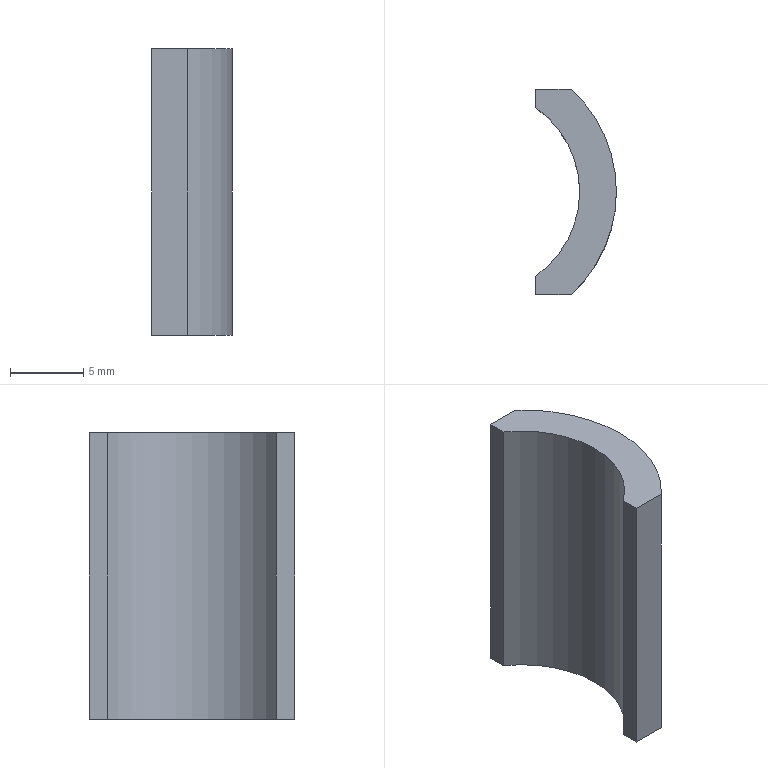Part | STEP file | magnet | 1 solid | 8 faces | box 5.5 x 14 x 19.5 mm | volume 770.904 mm3 | plane 6 | cylinder 2 | commonest cylinder face diameters 14 x1 19 x1
STEP:
#1=CARTESIAN_POINT('',(0.,0.,0.));
#2=DIRECTION('',(0.,0.,1.));
#3=DIRECTION('',(1.,0.,0.));
#4=AXIS2_PLACEMENT_3D('',#1,#2,#3);
#5=CARTESIAN_POINT('',(4.,-7.,0.));
#6=VERTEX_POINT('',#5);
#7=CARTESIAN_POINT('',(6.423,-7.,0.));
#8=VERTEX_POINT('',#7);
#9=CARTESIAN_POINT('',(4.,-7.,0.));
#10=DIRECTION('',(1.,0.,0.));
#11=VECTOR('',#10,1.);
#12=LINE('',#9,#11);
#13=CARTESIAN_POINT('',(4.,-7.,19.5));
#14=DIRECTION('',(0.,1.,0.));
#15=DIRECTION('',(-1.,0.,0.));
#16=AXIS2_PLACEMENT_3D('',#13,#14,#15);
#17=PLANE('',#16);
#18=CARTESIAN_POINT('',(0.,-19.5));
#19=DIRECTION('',(-1.,0.));
#20=VECTOR('',#19,1.);
#21=LINE('',#18,#20);
#22=(GEOMETRIC_REPRESENTATION_CONTEXT(2)PARAMETRIC_REPRESENTATION_CONTEXT()REPRESENTATION_CONTEXT('',''));
#23=DEFINITIONAL_REPRESENTATION('',(#21),#22);
#24=PCURVE('',#17,#23);
#25=CARTESIAN_POINT('',(0.,0.,0.));
#26=DIRECTION('',(0.,0.,1.));
#27=DIRECTION('',(1.,0.,0.));
#28=AXIS2_PLACEMENT_3D('',#25,#26,#27);
#29=PLANE('',#28);
#30=CARTESIAN_POINT('',(4.,-7.));
#31=DIRECTION('',(1.,0.));
#32=VECTOR('',#31,1.);
#33=LINE('',#30,#32);
#34=(GEOMETRIC_REPRESENTATION_CONTEXT(2)PARAMETRIC_REPRESENTATION_CONTEXT()REPRESENTATION_CONTEXT('',''));
#35=DEFINITIONAL_REPRESENTATION('',(#33),#34);
#36=PCURVE('',#29,#35);
#37=SURFACE_CURVE('',#12,(#24,#36),.PCURVE_S1.);
#38=EDGE_CURVE('',#6,#8,#37,.T.);
#39=ORIENTED_EDGE('',*,*,#38,.T.);
#40=CARTESIAN_POINT('',(6.423,-7.,19.5));
#41=VERTEX_POINT('',#40);
#42=CARTESIAN_POINT('',(6.423,-7.,19.5));
#43=DIRECTION('',(0.,0.,-1.));
#44=VECTOR('',#43,1.);
#45=LINE('',#42,#44);
#46=CARTESIAN_POINT('',(-2.423,0.));
#47=DIRECTION('',(0.,-1.));
#48=VECTOR('',#47,1.);
#49=LINE('',#46,#48);
#50=(GEOMETRIC_REPRESENTATION_CONTEXT(2)PARAMETRIC_REPRESENTATION_CONTEXT()REPRESENTATION_CONTEXT('',''));
#51=DEFINITIONAL_REPRESENTATION('',(#49),#50);
#52=PCURVE('',#17,#51);
#53=CARTESIAN_POINT('',(0.,0.,19.5));
#54=DIRECTION('',(0.,0.,-1.));
#55=DIRECTION('',(-1.,0.,0.));
#56=AXIS2_PLACEMENT_3D('',#53,#54,#55);
#57=CYLINDRICAL_SURFACE('',#56,9.5);
#58=CARTESIAN_POINT('',(3.97,0.));
#59=DIRECTION('',(0.,1.));
#60=VECTOR('',#59,1.);
#61=LINE('',#58,#60);
#62=(GEOMETRIC_REPRESENTATION_CONTEXT(2)PARAMETRIC_REPRESENTATION_CONTEXT()REPRESENTATION_CONTEXT('',''));
#63=DEFINITIONAL_REPRESENTATION('',(#61),#62);
#64=PCURVE('',#57,#63);
#65=SURFACE_CURVE('',#45,(#52,#64),.PCURVE_S1.);
#66=EDGE_CURVE('',#41,#8,#65,.T.);
#67=ORIENTED_EDGE('',*,*,#66,.F.);
#68=CARTESIAN_POINT('',(4.,-7.,19.5));
#69=VERTEX_POINT('',#68);
#70=CARTESIAN_POINT('',(4.,-7.,19.5));
#71=DIRECTION('',(1.,0.,0.));
#72=VECTOR('',#71,1.);
#73=LINE('',#70,#72);
#74=CARTESIAN_POINT('',(0.,0.));
#75=DIRECTION('',(-1.,0.));
#76=VECTOR('',#75,1.);
#77=LINE('',#74,#76);
#78=(GEOMETRIC_REPRESENTATION_CONTEXT(2)PARAMETRIC_REPRESENTATION_CONTEXT()REPRESENTATION_CONTEXT('',''));
#79=DEFINITIONAL_REPRESENTATION('',(#77),#78);
#80=PCURVE('',#17,#79);
#81=CARTESIAN_POINT('',(0.,0.,19.5));
#82=DIRECTION('',(0.,0.,1.));
#83=DIRECTION('',(1.,0.,0.));
#84=AXIS2_PLACEMENT_3D('',#81,#82,#83);
#85=PLANE('',#84);
#86=CARTESIAN_POINT('',(4.,-7.));
#87=DIRECTION('',(1.,0.));
#88=VECTOR('',#87,1.);
#89=LINE('',#86,#88);
#90=(GEOMETRIC_REPRESENTATION_CONTEXT(2)PARAMETRIC_REPRESENTATION_CONTEXT()REPRESENTATION_CONTEXT('',''));
#91=DEFINITIONAL_REPRESENTATION('',(#89),#90);
#92=PCURVE('',#85,#91);
#93=SURFACE_CURVE('',#73,(#80,#92),.PCURVE_S1.);
#94=EDGE_CURVE('',#69,#41,#93,.T.);
#95=ORIENTED_EDGE('',*,*,#94,.F.);
#96=CARTESIAN_POINT('',(4.,-7.,19.5));
#97=DIRECTION('',(0.,0.,-1.));
#98=VECTOR('',#97,1.);
#99=LINE('',#96,#98);
#100=CARTESIAN_POINT('',(0.,0.));
#101=DIRECTION('',(0.,-1.));
#102=VECTOR('',#101,1.);
#103=LINE('',#100,#102);
#104=(GEOMETRIC_REPRESENTATION_CONTEXT(2)PARAMETRIC_REPRESENTATION_CONTEXT()REPRESENTATION_CONTEXT('',''));
#105=DEFINITIONAL_REPRESENTATION('',(#103),#104);
#106=PCURVE('',#17,#105);
#107=CARTESIAN_POINT('',(4.,-7.,19.5));
#108=DIRECTION('',(1.,0.,0.));
#109=DIRECTION('',(0.,0.,-1.));
#110=AXIS2_PLACEMENT_3D('',#107,#108,#109);
#111=PLANE('',#110);
#112=CARTESIAN_POINT('',(0.,0.));
#113=DIRECTION('',(1.,0.));
#114=VECTOR('',#113,1.);
#115=LINE('',#112,#114);
#116=(GEOMETRIC_REPRESENTATION_CONTEXT(2)PARAMETRIC_REPRESENTATION_CONTEXT()REPRESENTATION_CONTEXT('',''));
#117=DEFINITIONAL_REPRESENTATION('',(#115),#116);
#118=PCURVE('',#111,#117);
#119=SURFACE_CURVE('',#99,(#106,#118),.PCURVE_S1.);
#120=EDGE_CURVE('',#69,#6,#119,.T.);
#121=ORIENTED_EDGE('',*,*,#120,.T.);
#122=EDGE_LOOP('',(#39,#67,#95,#121));
#123=FACE_BOUND('',#122,.T.);
#124=ADVANCED_FACE('',(#123),#17,.F.);
#125=CARTESIAN_POINT('',(6.423,7.,0.));
#126=VERTEX_POINT('',#125);
#127=CARTESIAN_POINT('',(0.,0.,0.));
#128=DIRECTION('',(0.,0.,1.));
#129=DIRECTION('',(1.,0.,0.));
#130=AXIS2_PLACEMENT_3D('',#127,#128,#129);
#131=CIRCLE('',#130,9.5);
#132=CARTESIAN_POINT('',(9.425,19.5));
#133=DIRECTION('',(-1.,0.));
#134=VECTOR('',#133,1.);
#135=LINE('',#132,#134);
#136=(GEOMETRIC_REPRESENTATION_CONTEXT(2)PARAMETRIC_REPRESENTATION_CONTEXT()REPRESENTATION_CONTEXT('',''));
#137=DEFINITIONAL_REPRESENTATION('',(#135),#136);
#138=PCURVE('',#57,#137);
#139=CARTESIAN_POINT('',(0.,0.));
#140=DIRECTION('',(1.,0.));
#141=AXIS2_PLACEMENT_2D('',#139,#140);
#142=CIRCLE('',#141,9.5);
#143=(GEOMETRIC_REPRESENTATION_CONTEXT(2)PARAMETRIC_REPRESENTATION_CONTEXT()REPRESENTATION_CONTEXT('',''));
#144=DEFINITIONAL_REPRESENTATION('',(#142),#143);
#145=PCURVE('',#29,#144);
#146=SURFACE_CURVE('',#131,(#138,#145),.PCURVE_S1.);
#147=EDGE_CURVE('',#8,#126,#146,.T.);
#148=ORIENTED_EDGE('',*,*,#147,.T.);
#149=CARTESIAN_POINT('',(6.423,7.,19.5));
#150=VERTEX_POINT('',#149);
#151=CARTESIAN_POINT('',(6.423,7.,19.5));
#152=DIRECTION('',(0.,0.,-1.));
#153=VECTOR('',#152,1.);
#154=LINE('',#151,#153);
#155=CARTESIAN_POINT('',(2.313,0.));
#156=DIRECTION('',(0.,1.));
#157=VECTOR('',#156,1.);
#158=LINE('',#155,#157);
#159=(GEOMETRIC_REPRESENTATION_CONTEXT(2)PARAMETRIC_REPRESENTATION_CONTEXT()REPRESENTATION_CONTEXT('',''));
#160=DEFINITIONAL_REPRESENTATION('',(#158),#159);
#161=PCURVE('',#57,#160);
#162=CARTESIAN_POINT('',(4.,7.,19.5));
#163=DIRECTION('',(0.,-1.,0.));
#164=DIRECTION('',(0.,0.,-1.));
#165=AXIS2_PLACEMENT_3D('',#162,#163,#164);
#166=PLANE('',#165);
#167=CARTESIAN_POINT('',(0.,2.423));
#168=DIRECTION('',(1.,0.));
#169=VECTOR('',#168,1.);
#170=LINE('',#167,#169);
#171=(GEOMETRIC_REPRESENTATION_CONTEXT(2)PARAMETRIC_REPRESENTATION_CONTEXT()REPRESENTATION_CONTEXT('',''));
#172=DEFINITIONAL_REPRESENTATION('',(#170),#171);
#173=PCURVE('',#166,#172);
#174=SURFACE_CURVE('',#154,(#161,#173),.PCURVE_S1.);
#175=EDGE_CURVE('',#150,#126,#174,.T.);
#176=ORIENTED_EDGE('',*,*,#175,.F.);
#177=CARTESIAN_POINT('',(0.,0.,19.5));
#178=DIRECTION('',(0.,0.,1.));
#179=DIRECTION('',(1.,0.,0.));
#180=AXIS2_PLACEMENT_3D('',#177,#178,#179);
#181=CIRCLE('',#180,9.5);
#182=CARTESIAN_POINT('',(9.425,0.));
#183=DIRECTION('',(-1.,0.));
#184=VECTOR('',#183,1.);
#185=LINE('',#182,#184);
#186=(GEOMETRIC_REPRESENTATION_CONTEXT(2)PARAMETRIC_REPRESENTATION_CONTEXT()REPRESENTATION_CONTEXT('',''));
#187=DEFINITIONAL_REPRESENTATION('',(#185),#186);
#188=PCURVE('',#57,#187);
#189=CARTESIAN_POINT('',(0.,0.));
#190=DIRECTION('',(1.,0.));
#191=AXIS2_PLACEMENT_2D('',#189,#190);
#192=CIRCLE('',#191,9.5);
#193=(GEOMETRIC_REPRESENTATION_CONTEXT(2)PARAMETRIC_REPRESENTATION_CONTEXT()REPRESENTATION_CONTEXT('',''));
#194=DEFINITIONAL_REPRESENTATION('',(#192),#193);
#195=PCURVE('',#85,#194);
#196=SURFACE_CURVE('',#181,(#188,#195),.PCURVE_S1.);
#197=EDGE_CURVE('',#41,#150,#196,.T.);
#198=ORIENTED_EDGE('',*,*,#197,.F.);
#199=ORIENTED_EDGE('',*,*,#66,.T.);
#200=EDGE_LOOP('',(#148,#176,#198,#199));
#201=FACE_BOUND('',#200,.T.);
#202=ADVANCED_FACE('',(#201),#57,.T.);
#203=CARTESIAN_POINT('',(4.,7.,0.));
#204=VERTEX_POINT('',#203);
#205=CARTESIAN_POINT('',(4.,7.,0.));
#206=DIRECTION('',(-1.,0.,0.));
#207=VECTOR('',#206,1.);
#208=LINE('',#205,#207);
#209=CARTESIAN_POINT('',(19.5,0.));
#210=DIRECTION('',(0.,-1.));
#211=VECTOR('',#210,1.);
#212=LINE('',#209,#211);
#213=(GEOMETRIC_REPRESENTATION_CONTEXT(2)PARAMETRIC_REPRESENTATION_CONTEXT()REPRESENTATION_CONTEXT('',''));
#214=DEFINITIONAL_REPRESENTATION('',(#212),#213);
#215=PCURVE('',#166,#214);
#216=CARTESIAN_POINT('',(4.,7.));
#217=DIRECTION('',(-1.,0.));
#218=VECTOR('',#217,1.);
#219=LINE('',#216,#218);
#220=(GEOMETRIC_REPRESENTATION_CONTEXT(2)PARAMETRIC_REPRESENTATION_CONTEXT()REPRESENTATION_CONTEXT('',''));
#221=DEFINITIONAL_REPRESENTATION('',(#219),#220);
#222=PCURVE('',#29,#221);
#223=SURFACE_CURVE('',#208,(#215,#222),.PCURVE_S1.);
#224=EDGE_CURVE('',#126,#204,#223,.T.);
#225=ORIENTED_EDGE('',*,*,#224,.T.);
#226=CARTESIAN_POINT('',(4.,7.,19.5));
#227=VERTEX_POINT('',#226);
#228=CARTESIAN_POINT('',(4.,7.,19.5));
#229=DIRECTION('',(0.,0.,-1.));
#230=VECTOR('',#229,1.);
#231=LINE('',#228,#230);
#232=CARTESIAN_POINT('',(0.,0.));
#233=DIRECTION('',(1.,0.));
#234=VECTOR('',#233,1.);
#235=LINE('',#232,#234);
#236=(GEOMETRIC_REPRESENTATION_CONTEXT(2)PARAMETRIC_REPRESENTATION_CONTEXT()REPRESENTATION_CONTEXT('',''));
#237=DEFINITIONAL_REPRESENTATION('',(#235),#236);
#238=PCURVE('',#166,#237);
#239=CARTESIAN_POINT('',(4.,5.745,19.5));
#240=DIRECTION('',(1.,0.,0.));
#241=DIRECTION('',(0.,0.,-1.));
#242=AXIS2_PLACEMENT_3D('',#239,#240,#241);
#243=PLANE('',#242);
#244=CARTESIAN_POINT('',(0.,1.255));
#245=DIRECTION('',(1.,0.));
#246=VECTOR('',#245,1.);
#247=LINE('',#244,#246);
#248=(GEOMETRIC_REPRESENTATION_CONTEXT(2)PARAMETRIC_REPRESENTATION_CONTEXT()REPRESENTATION_CONTEXT('',''));
#249=DEFINITIONAL_REPRESENTATION('',(#247),#248);
#250=PCURVE('',#243,#249);
#251=SURFACE_CURVE('',#231,(#238,#250),.PCURVE_S1.);
#252=EDGE_CURVE('',#227,#204,#251,.T.);
#253=ORIENTED_EDGE('',*,*,#252,.F.);
#254=CARTESIAN_POINT('',(4.,7.,19.5));
#255=DIRECTION('',(-1.,0.,0.));
#256=VECTOR('',#255,1.);
#257=LINE('',#254,#256);
#258=CARTESIAN_POINT('',(0.,0.));
#259=DIRECTION('',(0.,-1.));
#260=VECTOR('',#259,1.);
#261=LINE('',#258,#260);
#262=(GEOMETRIC_REPRESENTATION_CONTEXT(2)PARAMETRIC_REPRESENTATION_CONTEXT()REPRESENTATION_CONTEXT('',''));
#263=DEFINITIONAL_REPRESENTATION('',(#261),#262);
#264=PCURVE('',#166,#263);
#265=CARTESIAN_POINT('',(4.,7.));
#266=DIRECTION('',(-1.,0.));
#267=VECTOR('',#266,1.);
#268=LINE('',#265,#267);
#269=(GEOMETRIC_REPRESENTATION_CONTEXT(2)PARAMETRIC_REPRESENTATION_CONTEXT()REPRESENTATION_CONTEXT('',''));
#270=DEFINITIONAL_REPRESENTATION('',(#268),#269);
#271=PCURVE('',#85,#270);
#272=SURFACE_CURVE('',#257,(#264,#271),.PCURVE_S1.);
#273=EDGE_CURVE('',#150,#227,#272,.T.);
#274=ORIENTED_EDGE('',*,*,#273,.F.);
#275=ORIENTED_EDGE('',*,*,#175,.T.);
#276=EDGE_LOOP('',(#225,#253,#274,#275));
#277=FACE_BOUND('',#276,.T.);
#278=ADVANCED_FACE('',(#277),#166,.F.);
#279=CARTESIAN_POINT('',(4.,5.745,0.));
#280=VERTEX_POINT('',#279);
#281=CARTESIAN_POINT('',(4.,5.745,0.));
#282=DIRECTION('',(0.,-1.,0.));
#283=VECTOR('',#282,1.);
#284=LINE('',#281,#283);
#285=CARTESIAN_POINT('',(19.5,0.));
#286=DIRECTION('',(0.,-1.));
#287=VECTOR('',#286,1.);
#288=LINE('',#285,#287);
#289=(GEOMETRIC_REPRESENTATION_CONTEXT(2)PARAMETRIC_REPRESENTATION_CONTEXT()REPRESENTATION_CONTEXT('',''));
#290=DEFINITIONAL_REPRESENTATION('',(#288),#289);
#291=PCURVE('',#243,#290);
#292=CARTESIAN_POINT('',(4.,5.745));
#293=DIRECTION('',(0.,-1.));
#294=VECTOR('',#293,1.);
#295=LINE('',#292,#294);
#296=(GEOMETRIC_REPRESENTATION_CONTEXT(2)PARAMETRIC_REPRESENTATION_CONTEXT()REPRESENTATION_CONTEXT('',''));
#297=DEFINITIONAL_REPRESENTATION('',(#295),#296);
#298=PCURVE('',#29,#297);
#299=SURFACE_CURVE('',#284,(#291,#298),.PCURVE_S1.);
#300=EDGE_CURVE('',#204,#280,#299,.T.);
#301=ORIENTED_EDGE('',*,*,#300,.T.);
#302=CARTESIAN_POINT('',(4.,5.745,19.5));
#303=VERTEX_POINT('',#302);
#304=CARTESIAN_POINT('',(4.,5.745,19.5));
#305=DIRECTION('',(0.,0.,-1.));
#306=VECTOR('',#305,1.);
#307=LINE('',#304,#306);
#308=CARTESIAN_POINT('',(0.,0.));
#309=DIRECTION('',(1.,0.));
#310=VECTOR('',#309,1.);
#311=LINE('',#308,#310);
#312=(GEOMETRIC_REPRESENTATION_CONTEXT(2)PARAMETRIC_REPRESENTATION_CONTEXT()REPRESENTATION_CONTEXT('',''));
#313=DEFINITIONAL_REPRESENTATION('',(#311),#312);
#314=PCURVE('',#243,#313);
#315=CARTESIAN_POINT('',(0.,0.,19.5));
#316=DIRECTION('',(0.,0.,-1.));
#317=DIRECTION('',(-1.,0.,0.));
#318=AXIS2_PLACEMENT_3D('',#315,#316,#317);
#319=CYLINDRICAL_SURFACE('',#318,7.);
#320=CARTESIAN_POINT('',(2.179,0.));
#321=DIRECTION('',(0.,1.));
#322=VECTOR('',#321,1.);
#323=LINE('',#320,#322);
#324=(GEOMETRIC_REPRESENTATION_CONTEXT(2)PARAMETRIC_REPRESENTATION_CONTEXT()REPRESENTATION_CONTEXT('',''));
#325=DEFINITIONAL_REPRESENTATION('',(#323),#324);
#326=PCURVE('',#319,#325);
#327=SURFACE_CURVE('',#307,(#314,#326),.PCURVE_S1.);
#328=EDGE_CURVE('',#303,#280,#327,.T.);
#329=ORIENTED_EDGE('',*,*,#328,.F.);
#330=CARTESIAN_POINT('',(4.,5.745,19.5));
#331=DIRECTION('',(0.,-1.,0.));
#332=VECTOR('',#331,1.);
#333=LINE('',#330,#332);
#334=CARTESIAN_POINT('',(0.,0.));
#335=DIRECTION('',(0.,-1.));
#336=VECTOR('',#335,1.);
#337=LINE('',#334,#336);
#338=(GEOMETRIC_REPRESENTATION_CONTEXT(2)PARAMETRIC_REPRESENTATION_CONTEXT()REPRESENTATION_CONTEXT('',''));
#339=DEFINITIONAL_REPRESENTATION('',(#337),#338);
#340=PCURVE('',#243,#339);
#341=CARTESIAN_POINT('',(4.,5.745));
#342=DIRECTION('',(0.,-1.));
#343=VECTOR('',#342,1.);
#344=LINE('',#341,#343);
#345=(GEOMETRIC_REPRESENTATION_CONTEXT(2)PARAMETRIC_REPRESENTATION_CONTEXT()REPRESENTATION_CONTEXT('',''));
#346=DEFINITIONAL_REPRESENTATION('',(#344),#345);
#347=PCURVE('',#85,#346);
#348=SURFACE_CURVE('',#333,(#340,#347),.PCURVE_S1.);
#349=EDGE_CURVE('',#227,#303,#348,.T.);
#350=ORIENTED_EDGE('',*,*,#349,.F.);
#351=ORIENTED_EDGE('',*,*,#252,.T.);
#352=EDGE_LOOP('',(#301,#329,#350,#351));
#353=FACE_BOUND('',#352,.T.);
#354=ADVANCED_FACE('',(#353),#243,.F.);
#355=ORIENTED_EDGE('',*,*,#328,.F.);
#356=CARTESIAN_POINT('',(4.,-5.745,19.5));
#357=VERTEX_POINT('',#356);
#358=CARTESIAN_POINT('',(0.,0.,19.5));
#359=DIRECTION('',(0.,0.,-1.));
#360=DIRECTION('',(1.,0.,0.));
#361=AXIS2_PLACEMENT_3D('',#358,#359,#360);
#362=CIRCLE('',#361,7.);
#363=CARTESIAN_POINT('',(-3.142,0.));
#364=DIRECTION('',(1.,0.));
#365=VECTOR('',#364,1.);
#366=LINE('',#363,#365);
#367=(GEOMETRIC_REPRESENTATION_CONTEXT(2)PARAMETRIC_REPRESENTATION_CONTEXT()REPRESENTATION_CONTEXT('',''));
#368=DEFINITIONAL_REPRESENTATION('',(#366),#367);
#369=PCURVE('',#319,#368);
#370=CARTESIAN_POINT('',(7.,0.));
#371=CARTESIAN_POINT('',(7.,-12.124));
#372=CARTESIAN_POINT('',(-3.5,-6.062));
#373=CARTESIAN_POINT('',(-14.,0.));
#374=CARTESIAN_POINT('',(-3.5,6.062));
#375=CARTESIAN_POINT('',(7.,12.124));
#376=CARTESIAN_POINT('',(7.,0.));
#377=(BOUNDED_CURVE()B_SPLINE_CURVE(2,(#370,#371,#372,#373,#374,#375,#376),.UNSPECIFIED.,.T.,.F.)B_SPLINE_CURVE_WITH_KNOTS((1,2,2,2,2,1),(-2.094,0.,2.094,4.189,6.283,8.378),.UNSPECIFIED.)CURVE()GEOMETRIC_REPRESENTATION_ITEM()RATIONAL_B_SPLINE_CURVE((1.,0.5,1.,0.5,1.,0.5,1.))REPRESENTATION_ITEM(''));
#378=(GEOMETRIC_REPRESENTATION_CONTEXT(2)PARAMETRIC_REPRESENTATION_CONTEXT()REPRESENTATION_CONTEXT('',''));
#379=DEFINITIONAL_REPRESENTATION('',(#377),#378);
#380=PCURVE('',#85,#379);
#381=SURFACE_CURVE('',#362,(#369,#380),.PCURVE_S1.);
#382=EDGE_CURVE('',#303,#357,#381,.T.);
#383=ORIENTED_EDGE('',*,*,#382,.T.);
#384=CARTESIAN_POINT('',(4.,-5.745,0.));
#385=VERTEX_POINT('',#384);
#386=CARTESIAN_POINT('',(4.,-5.745,19.5));
#387=DIRECTION('',(0.,0.,-1.));
#388=VECTOR('',#387,1.);
#389=LINE('',#386,#388);
#390=CARTESIAN_POINT('',(4.104,0.));
#391=DIRECTION('',(0.,1.));
#392=VECTOR('',#391,1.);
#393=LINE('',#390,#392);
#394=(GEOMETRIC_REPRESENTATION_CONTEXT(2)PARAMETRIC_REPRESENTATION_CONTEXT()REPRESENTATION_CONTEXT('',''));
#395=DEFINITIONAL_REPRESENTATION('',(#393),#394);
#396=PCURVE('',#319,#395);
#397=CARTESIAN_POINT('',(0.,1.255));
#398=DIRECTION('',(1.,0.));
#399=VECTOR('',#398,1.);
#400=LINE('',#397,#399);
#401=(GEOMETRIC_REPRESENTATION_CONTEXT(2)PARAMETRIC_REPRESENTATION_CONTEXT()REPRESENTATION_CONTEXT('',''));
#402=DEFINITIONAL_REPRESENTATION('',(#400),#401);
#403=PCURVE('',#111,#402);
#404=SURFACE_CURVE('',#389,(#396,#403),.PCURVE_S1.);
#405=EDGE_CURVE('',#357,#385,#404,.T.);
#406=ORIENTED_EDGE('',*,*,#405,.T.);
#407=CARTESIAN_POINT('',(0.,0.,0.));
#408=DIRECTION('',(0.,0.,-1.));
#409=DIRECTION('',(1.,0.,0.));
#410=AXIS2_PLACEMENT_3D('',#407,#408,#409);
#411=CIRCLE('',#410,7.);
#412=CARTESIAN_POINT('',(-3.142,19.5));
#413=DIRECTION('',(1.,0.));
#414=VECTOR('',#413,1.);
#415=LINE('',#412,#414);
#416=(GEOMETRIC_REPRESENTATION_CONTEXT(2)PARAMETRIC_REPRESENTATION_CONTEXT()REPRESENTATION_CONTEXT('',''));
#417=DEFINITIONAL_REPRESENTATION('',(#415),#416);
#418=PCURVE('',#319,#417);
#419=CARTESIAN_POINT('',(7.,0.));
#420=CARTESIAN_POINT('',(7.,-12.124));
#421=CARTESIAN_POINT('',(-3.5,-6.062));
#422=CARTESIAN_POINT('',(-14.,0.));
#423=CARTESIAN_POINT('',(-3.5,6.062));
#424=CARTESIAN_POINT('',(7.,12.124));
#425=CARTESIAN_POINT('',(7.,0.));
#426=(BOUNDED_CURVE()B_SPLINE_CURVE(2,(#419,#420,#421,#422,#423,#424,#425),.UNSPECIFIED.,.T.,.F.)B_SPLINE_CURVE_WITH_KNOTS((1,2,2,2,2,1),(-2.094,0.,2.094,4.189,6.283,8.378),.UNSPECIFIED.)CURVE()GEOMETRIC_REPRESENTATION_ITEM()RATIONAL_B_SPLINE_CURVE((1.,0.5,1.,0.5,1.,0.5,1.))REPRESENTATION_ITEM(''));
#427=(GEOMETRIC_REPRESENTATION_CONTEXT(2)PARAMETRIC_REPRESENTATION_CONTEXT()REPRESENTATION_CONTEXT('',''));
#428=DEFINITIONAL_REPRESENTATION('',(#426),#427);
#429=PCURVE('',#29,#428);
#430=SURFACE_CURVE('',#411,(#418,#429),.PCURVE_S1.);
#431=EDGE_CURVE('',#280,#385,#430,.T.);
#432=ORIENTED_EDGE('',*,*,#431,.F.);
#433=EDGE_LOOP('',(#355,#383,#406,#432));
#434=FACE_BOUND('',#433,.F.);
#435=ADVANCED_FACE('',(#434),#319,.F.);
#436=CARTESIAN_POINT('',(4.,-7.,0.));
#437=DIRECTION('',(0.,-1.,0.));
#438=VECTOR('',#437,1.);
#439=LINE('',#436,#438);
#440=CARTESIAN_POINT('',(19.5,0.));
#441=DIRECTION('',(0.,-1.));
#442=VECTOR('',#441,1.);
#443=LINE('',#440,#442);
#444=(GEOMETRIC_REPRESENTATION_CONTEXT(2)PARAMETRIC_REPRESENTATION_CONTEXT()REPRESENTATION_CONTEXT('',''));
#445=DEFINITIONAL_REPRESENTATION('',(#443),#444);
#446=PCURVE('',#111,#445);
#447=CARTESIAN_POINT('',(4.,-7.));
#448=DIRECTION('',(0.,-1.));
#449=VECTOR('',#448,1.);
#450=LINE('',#447,#449);
#451=(GEOMETRIC_REPRESENTATION_CONTEXT(2)PARAMETRIC_REPRESENTATION_CONTEXT()REPRESENTATION_CONTEXT('',''));
#452=DEFINITIONAL_REPRESENTATION('',(#450),#451);
#453=PCURVE('',#29,#452);
#454=SURFACE_CURVE('',#439,(#446,#453),.PCURVE_S1.);
#455=EDGE_CURVE('',#385,#6,#454,.T.);
#456=ORIENTED_EDGE('',*,*,#455,.T.);
#457=ORIENTED_EDGE('',*,*,#120,.F.);
#458=CARTESIAN_POINT('',(4.,-7.,19.5));
#459=DIRECTION('',(0.,-1.,0.));
#460=VECTOR('',#459,1.);
#461=LINE('',#458,#460);
#462=CARTESIAN_POINT('',(0.,0.));
#463=DIRECTION('',(0.,-1.));
#464=VECTOR('',#463,1.);
#465=LINE('',#462,#464);
#466=(GEOMETRIC_REPRESENTATION_CONTEXT(2)PARAMETRIC_REPRESENTATION_CONTEXT()REPRESENTATION_CONTEXT('',''));
#467=DEFINITIONAL_REPRESENTATION('',(#465),#466);
#468=PCURVE('',#111,#467);
#469=CARTESIAN_POINT('',(4.,-7.));
#470=DIRECTION('',(0.,-1.));
#471=VECTOR('',#470,1.);
#472=LINE('',#469,#471);
#473=(GEOMETRIC_REPRESENTATION_CONTEXT(2)PARAMETRIC_REPRESENTATION_CONTEXT()REPRESENTATION_CONTEXT('',''));
#474=DEFINITIONAL_REPRESENTATION('',(#472),#473);
#475=PCURVE('',#85,#474);
#476=SURFACE_CURVE('',#461,(#468,#475),.PCURVE_S1.);
#477=EDGE_CURVE('',#357,#69,#476,.T.);
#478=ORIENTED_EDGE('',*,*,#477,.F.);
#479=ORIENTED_EDGE('',*,*,#405,.T.);
#480=EDGE_LOOP('',(#456,#457,#478,#479));
#481=FACE_BOUND('',#480,.T.);
#482=ADVANCED_FACE('',(#481),#111,.F.);
#483=ORIENTED_EDGE('',*,*,#94,.T.);
#484=ORIENTED_EDGE('',*,*,#197,.T.);
#485=ORIENTED_EDGE('',*,*,#273,.T.);
#486=ORIENTED_EDGE('',*,*,#349,.T.);
#487=ORIENTED_EDGE('',*,*,#382,.T.);
#488=ORIENTED_EDGE('',*,*,#477,.T.);
#489=EDGE_LOOP('',(#483,#484,#485,#486,#487,#488));
#490=FACE_BOUND('',#489,.T.);
#491=ADVANCED_FACE('',(#490),#85,.T.);
#492=ORIENTED_EDGE('',*,*,#38,.F.);
#493=ORIENTED_EDGE('',*,*,#455,.F.);
#494=ORIENTED_EDGE('',*,*,#431,.F.);
#495=ORIENTED_EDGE('',*,*,#300,.F.);
#496=ORIENTED_EDGE('',*,*,#224,.F.);
#497=ORIENTED_EDGE('',*,*,#147,.F.);
#498=EDGE_LOOP('',(#492,#493,#494,#495,#496,#497));
#499=FACE_BOUND('',#498,.T.);
#500=ADVANCED_FACE('',(#499),#29,.F.);
#501=CLOSED_SHELL('',(#124,#202,#278,#354,#435,#482,#491,#500));
#502=MANIFOLD_SOLID_BREP('',#501);
#503=(LENGTH_UNIT()NAMED_UNIT(*)SI_UNIT(.MILLI.,.METRE.));
#504=UNCERTAINTY_MEASURE_WITH_UNIT(LENGTH_MEASURE(0.0000001),#503,'','');
#505=(NAMED_UNIT(*)PLANE_ANGLE_UNIT()SI_UNIT($,.RADIAN.));
#506=(NAMED_UNIT(*)SI_UNIT($,.STERADIAN.)SOLID_ANGLE_UNIT());
#507=(GEOMETRIC_REPRESENTATION_CONTEXT(3)GLOBAL_UNCERTAINTY_ASSIGNED_CONTEXT((#504))GLOBAL_UNIT_ASSIGNED_CONTEXT((#503,#505,#506))REPRESENTATION_CONTEXT('',''));
#508=ADVANCED_BREP_SHAPE_REPRESENTATION('',(#4,#502),#507);